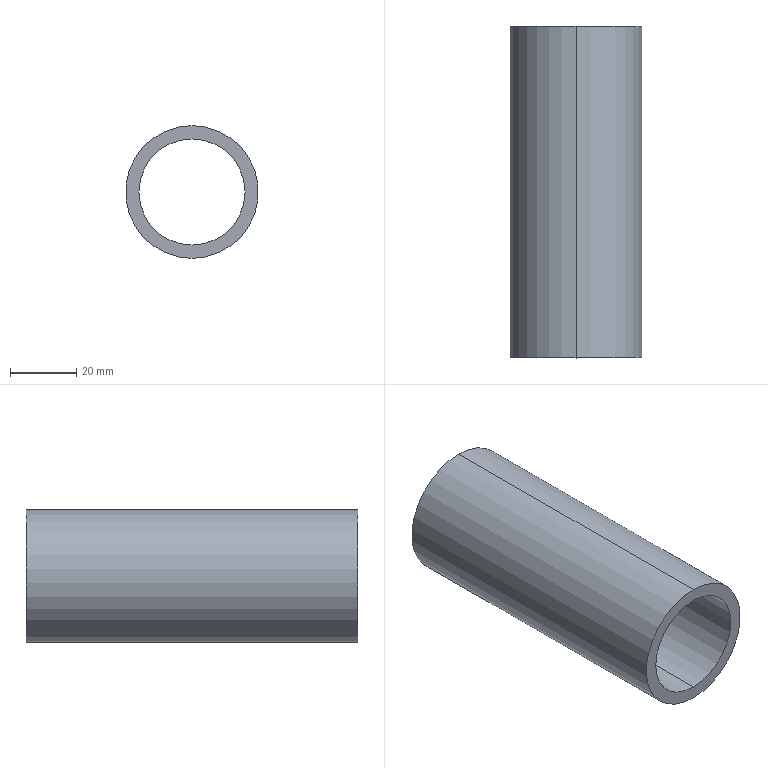Part | STEP file | inner cylinder block | 1 solid | 6 faces | box 40 x 100 x 40 mm | volume 45239 mm3 | cylinder 4 | plane 2 | commonest cylinder face diameters 32 x2 40 x2
STEP:
#1=CARTESIAN_POINT('',(0.,-50.,20.));
#2=VERTEX_POINT('',#1);
#3=CARTESIAN_POINT('',(0.,-50.,-20.));
#4=VERTEX_POINT('',#3);
#5=CARTESIAN_POINT('',(0.,-50.,0.));
#6=DIRECTION('',(0.,1.,0.));
#7=DIRECTION('',(0.,0.,1.));
#8=AXIS2_PLACEMENT_3D('',#5,#6,#7);
#9=CIRCLE('',#8,20.);
#10=EDGE_CURVE('',#2,#4,#9,.T.);
#11=ORIENTED_EDGE('',*,*,#10,.T.);
#12=CARTESIAN_POINT('',(0.,50.,-20.));
#13=VERTEX_POINT('',#12);
#14=CARTESIAN_POINT('',(0.,26.149,-20.));
#15=DIRECTION('',(0.,1.,0.));
#16=VECTOR('',#15,1000.);
#17=LINE('',#14,#16);
#18=EDGE_CURVE('',#4,#13,#17,.T.);
#19=ORIENTED_EDGE('',*,*,#18,.T.);
#20=CARTESIAN_POINT('',(0.,50.,20.));
#21=VERTEX_POINT('',#20);
#22=CARTESIAN_POINT('',(0.,50.,0.));
#23=DIRECTION('',(0.,1.,0.));
#24=DIRECTION('',(0.,0.,1.));
#25=AXIS2_PLACEMENT_3D('',#22,#23,#24);
#26=CIRCLE('',#25,20.);
#27=EDGE_CURVE('',#21,#13,#26,.T.);
#28=ORIENTED_EDGE('',*,*,#27,.F.);
#29=CARTESIAN_POINT('',(0.,26.149,20.));
#30=DIRECTION('',(0.,1.,0.));
#31=VECTOR('',#30,1000.);
#32=LINE('',#29,#31);
#33=EDGE_CURVE('',#2,#21,#32,.T.);
#34=ORIENTED_EDGE('',*,*,#33,.F.);
#35=EDGE_LOOP('',(#11,#19,#28,#34));
#36=FACE_OUTER_BOUND('',#35,.T.);
#37=CARTESIAN_POINT('',(0.,26.149,0.));
#38=DIRECTION('',(0.,1.,0.));
#39=DIRECTION('',(0.,0.,1.));
#40=AXIS2_PLACEMENT_3D('',#37,#38,#39);
#41=CYLINDRICAL_SURFACE('',#40,20.);
#42=ADVANCED_FACE('',(#36),#41,.T.);
#43=CARTESIAN_POINT('',(0.,-50.,-16.));
#44=VERTEX_POINT('',#43);
#45=CARTESIAN_POINT('',(0.,-50.,16.));
#46=VERTEX_POINT('',#45);
#47=CARTESIAN_POINT('',(0.,-50.,0.));
#48=DIRECTION('',(0.,1.,0.));
#49=DIRECTION('',(0.,0.,1.));
#50=AXIS2_PLACEMENT_3D('',#47,#48,#49);
#51=CIRCLE('',#50,16.);
#52=EDGE_CURVE('',#44,#46,#51,.T.);
#53=ORIENTED_EDGE('',*,*,#52,.F.);
#54=CARTESIAN_POINT('',(0.,50.,-16.));
#55=VERTEX_POINT('',#54);
#56=CARTESIAN_POINT('',(0.,26.149,-16.));
#57=DIRECTION('',(0.,1.,0.));
#58=VECTOR('',#57,1000.);
#59=LINE('',#56,#58);
#60=EDGE_CURVE('',#44,#55,#59,.T.);
#61=ORIENTED_EDGE('',*,*,#60,.T.);
#62=CARTESIAN_POINT('',(0.,50.,16.));
#63=VERTEX_POINT('',#62);
#64=CARTESIAN_POINT('',(0.,50.,0.));
#65=DIRECTION('',(0.,1.,0.));
#66=DIRECTION('',(0.,0.,1.));
#67=AXIS2_PLACEMENT_3D('',#64,#65,#66);
#68=CIRCLE('',#67,16.);
#69=EDGE_CURVE('',#55,#63,#68,.T.);
#70=ORIENTED_EDGE('',*,*,#69,.T.);
#71=CARTESIAN_POINT('',(0.,26.149,16.));
#72=DIRECTION('',(0.,1.,0.));
#73=VECTOR('',#72,1000.);
#74=LINE('',#71,#73);
#75=EDGE_CURVE('',#46,#63,#74,.T.);
#76=ORIENTED_EDGE('',*,*,#75,.F.);
#77=EDGE_LOOP('',(#53,#61,#70,#76));
#78=FACE_OUTER_BOUND('',#77,.T.);
#79=CARTESIAN_POINT('',(0.,26.149,0.));
#80=DIRECTION('',(0.,1.,0.));
#81=DIRECTION('',(0.,0.,1.));
#82=AXIS2_PLACEMENT_3D('',#79,#80,#81);
#83=CYLINDRICAL_SURFACE('',#82,16.);
#84=ADVANCED_FACE('',(#78),#83,.F.);
#85=ORIENTED_EDGE('',*,*,#60,.F.);
#86=CARTESIAN_POINT('',(0.,-50.,0.));
#87=DIRECTION('',(0.,1.,0.));
#88=DIRECTION('',(0.,0.,1.));
#89=AXIS2_PLACEMENT_3D('',#86,#87,#88);
#90=CIRCLE('',#89,16.);
#91=EDGE_CURVE('',#46,#44,#90,.T.);
#92=ORIENTED_EDGE('',*,*,#91,.F.);
#93=ORIENTED_EDGE('',*,*,#75,.T.);
#94=CARTESIAN_POINT('',(0.,50.,0.));
#95=DIRECTION('',(0.,1.,0.));
#96=DIRECTION('',(0.,0.,1.));
#97=AXIS2_PLACEMENT_3D('',#94,#95,#96);
#98=CIRCLE('',#97,16.);
#99=EDGE_CURVE('',#63,#55,#98,.T.);
#100=ORIENTED_EDGE('',*,*,#99,.T.);
#101=EDGE_LOOP('',(#85,#92,#93,#100));
#102=FACE_OUTER_BOUND('',#101,.T.);
#103=CARTESIAN_POINT('',(0.,26.149,0.));
#104=DIRECTION('',(0.,1.,0.));
#105=DIRECTION('',(0.,0.,1.));
#106=AXIS2_PLACEMENT_3D('',#103,#104,#105);
#107=CYLINDRICAL_SURFACE('',#106,16.);
#108=ADVANCED_FACE('',(#102),#107,.F.);
#109=ORIENTED_EDGE('',*,*,#27,.T.);
#110=CARTESIAN_POINT('',(0.,50.,0.));
#111=DIRECTION('',(0.,1.,0.));
#112=DIRECTION('',(0.,0.,1.));
#113=AXIS2_PLACEMENT_3D('',#110,#111,#112);
#114=CIRCLE('',#113,20.);
#115=EDGE_CURVE('',#13,#21,#114,.T.);
#116=ORIENTED_EDGE('',*,*,#115,.T.);
#117=EDGE_LOOP('',(#109,#116));
#118=FACE_OUTER_BOUND('',#117,.T.);
#119=ORIENTED_EDGE('',*,*,#99,.F.);
#120=ORIENTED_EDGE('',*,*,#69,.F.);
#121=EDGE_LOOP('',(#119,#120));
#122=FACE_BOUND('',#121,.T.);
#123=CARTESIAN_POINT('',(-20.,50.,0.));
#124=DIRECTION('',(0.,1.,0.));
#125=DIRECTION('',(0.,0.,1.));
#126=AXIS2_PLACEMENT_3D('',#123,#124,#125);
#127=PLANE('',#126);
#128=ADVANCED_FACE('',(#118,#122),#127,.T.);
#129=ORIENTED_EDGE('',*,*,#18,.F.);
#130=CARTESIAN_POINT('',(0.,-50.,0.));
#131=DIRECTION('',(0.,1.,0.));
#132=DIRECTION('',(0.,0.,1.));
#133=AXIS2_PLACEMENT_3D('',#130,#131,#132);
#134=CIRCLE('',#133,20.);
#135=EDGE_CURVE('',#4,#2,#134,.T.);
#136=ORIENTED_EDGE('',*,*,#135,.T.);
#137=ORIENTED_EDGE('',*,*,#33,.T.);
#138=ORIENTED_EDGE('',*,*,#115,.F.);
#139=EDGE_LOOP('',(#129,#136,#137,#138));
#140=FACE_OUTER_BOUND('',#139,.T.);
#141=CARTESIAN_POINT('',(0.,26.149,0.));
#142=DIRECTION('',(0.,1.,0.));
#143=DIRECTION('',(0.,0.,1.));
#144=AXIS2_PLACEMENT_3D('',#141,#142,#143);
#145=CYLINDRICAL_SURFACE('',#144,20.);
#146=ADVANCED_FACE('',(#140),#145,.T.);
#147=ORIENTED_EDGE('',*,*,#91,.T.);
#148=ORIENTED_EDGE('',*,*,#52,.T.);
#149=EDGE_LOOP('',(#147,#148));
#150=FACE_BOUND('',#149,.T.);
#151=ORIENTED_EDGE('',*,*,#10,.F.);
#152=ORIENTED_EDGE('',*,*,#135,.F.);
#153=EDGE_LOOP('',(#151,#152));
#154=FACE_OUTER_BOUND('',#153,.T.);
#155=CARTESIAN_POINT('',(-20.,-50.,0.));
#156=DIRECTION('',(0.,-1.,0.));
#157=DIRECTION('',(0.,0.,-1.));
#158=AXIS2_PLACEMENT_3D('',#155,#156,#157);
#159=PLANE('',#158);
#160=ADVANCED_FACE('',(#150,#154),#159,.T.);
#161=CLOSED_SHELL('',(#42,#84,#108,#128,#146,#160));
#162=MANIFOLD_SOLID_BREP('',#161);
#163=CARTESIAN_POINT('',(0.,0.,0.));
#164=DIRECTION('',(0.,0.,1.));
#165=DIRECTION('',(1.,0.,0.));
#166=AXIS2_PLACEMENT_3D('',#163,#164,#165);
#167=(LENGTH_UNIT()NAMED_UNIT(*)SI_UNIT(.MILLI.,.METRE.));
#168=UNCERTAINTY_MEASURE_WITH_UNIT(LENGTH_MEASURE(0.00001),#167,'','');
#169=(NAMED_UNIT(*)PLANE_ANGLE_UNIT()SI_UNIT($,.RADIAN.));
#170=(NAMED_UNIT(*)SI_UNIT($,.STERADIAN.)SOLID_ANGLE_UNIT());
#171=(GEOMETRIC_REPRESENTATION_CONTEXT(3)GLOBAL_UNCERTAINTY_ASSIGNED_CONTEXT((#168))GLOBAL_UNIT_ASSIGNED_CONTEXT((#167,#169,#170))REPRESENTATION_CONTEXT('',''));
#172=ADVANCED_BREP_SHAPE_REPRESENTATION('',(#162,#166),#171);